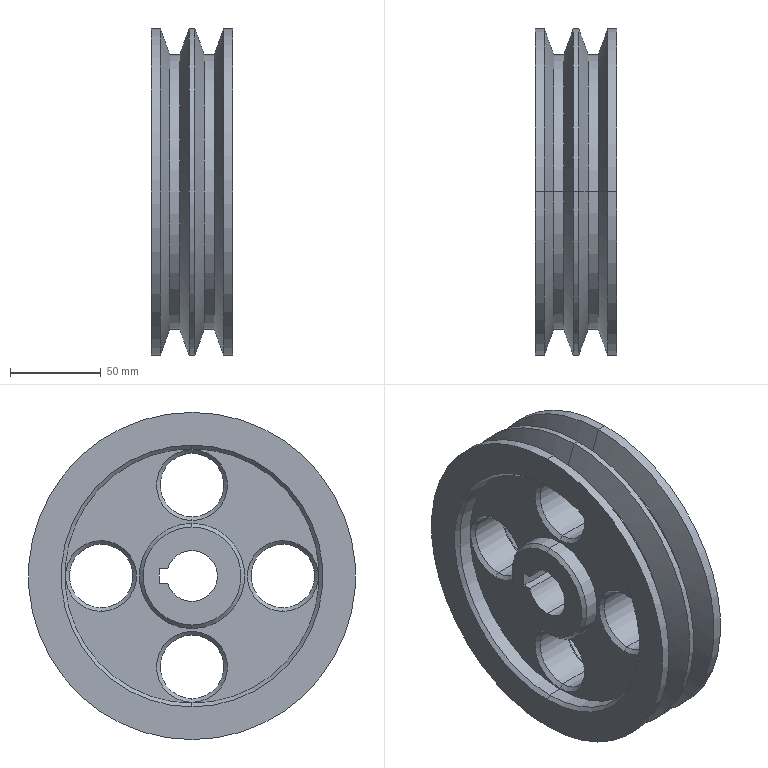Part | STEP file | Produce dryer line heating fan-PULLY-B-2-150 | 1 solid | 70 faces | box 45 x 180 x 180 mm | volume 597383 mm3 | cone 32 | cylinder 29 | plane 9 | commonest cylinder face diameters 35 x8 180 x6 58 x4 140 x4 151.4 x4 28 x3